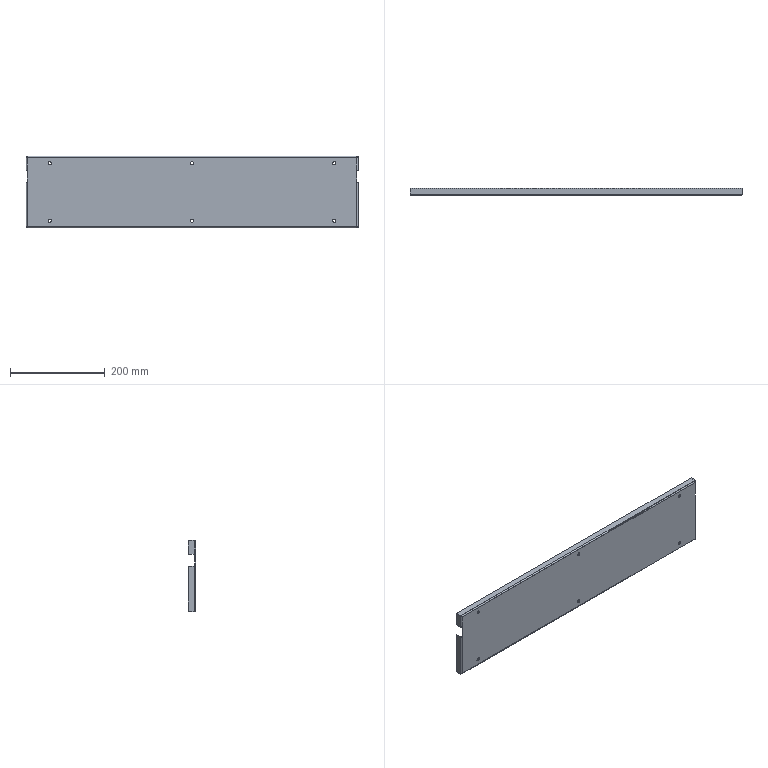Part | STEP file | 1 solid | 82 faces | box 700 x 15 x 151 mm | volume 151826 mm3 | plane 58 | cylinder 24 | commonest cylinder face diameters 7 x12 3 x6 5.4 x6